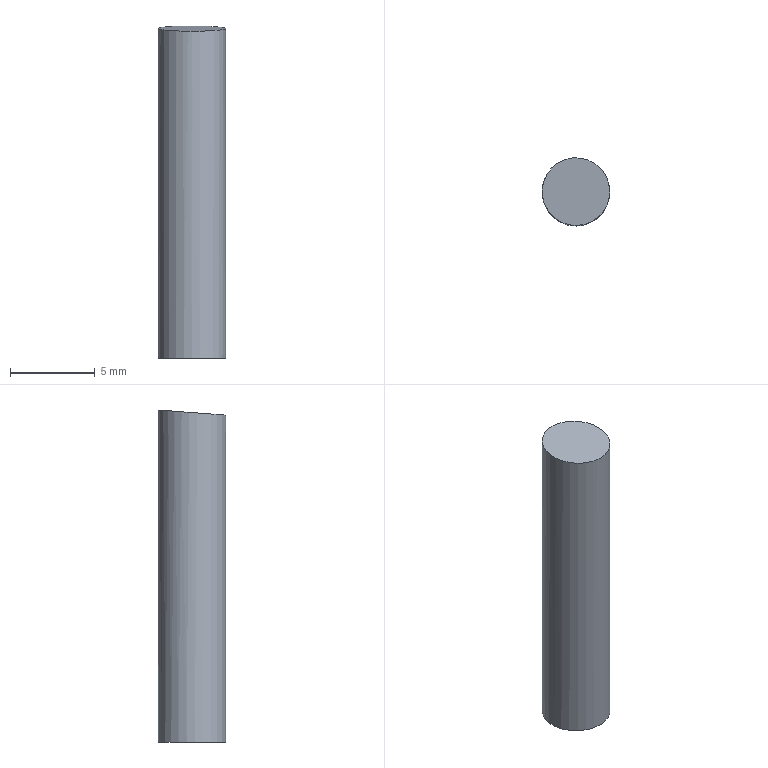Part | NX | features solid 2 | 1 solid | 3 faces | box 4 x 4 x 19.611 mm | volume 244.499 mm3 | plane 2 | cylinder 1 | commonest cylinder face diameters 4 x1
STEP:
#1=CARTESIAN_POINT('',(327.26,-25.675,-35.5));
#2=VERTEX_POINT('',#1);
#3=CARTESIAN_POINT('',(325.26,-25.675,-35.5));
#4=DIRECTION('',(0.,0.,1.));
#5=DIRECTION('',(1.,0.,0.));
#6=AXIS2_PLACEMENT_3D('',#3,#4,#5);
#7=CIRCLE('',#6,2.);
#8=EDGE_CURVE('',#2,#2,#7,.T.);
#9=ORIENTED_EDGE('',*,*,#8,.F.);
#10=EDGE_LOOP('',(#9));
#11=FACE_BOUND('',#10,.T.);
#12=CARTESIAN_POINT('',(325.26,-25.675,-35.5));
#13=DIRECTION('',(0.,0.,-1.));
#14=DIRECTION('',(-1.,0.,0.));
#15=AXIS2_PLACEMENT_3D('',#12,#13,#14);
#16=PLANE('',#15);
#17=ADVANCED_FACE('',(#11),#16,.T.);
#18=CARTESIAN_POINT('',(325.279,-27.675,-16.197));
#19=VERTEX_POINT('',#18);
#20=CARTESIAN_POINT('',(325.26,-25.675,-16.043));
#21=DIRECTION('',(0.0007587,-0.07675,0.9971));
#22=DIRECTION('',(0.009856,-0.997,-0.07675));
#23=AXIS2_PLACEMENT_3D('',#20,#21,#22);
#24=ELLIPSE('',#23,2.006,2.);
#25=EDGE_CURVE('',#19,#19,#24,.F.);
#26=ORIENTED_EDGE('',*,*,#25,.F.);
#27=EDGE_LOOP('',(#26));
#28=FACE_BOUND('',#27,.T.);
#29=CARTESIAN_POINT('',(464.929,116.723,-5.189));
#30=DIRECTION('',(0.0007587,-0.07675,0.9971));
#31=DIRECTION('',(-1.,0.004401,0.0011));
#32=AXIS2_PLACEMENT_3D('',#29,#30,#31);
#33=PLANE('',#32);
#34=ADVANCED_FACE('',(#28),#33,.T.);
#35=ORIENTED_EDGE('',*,*,#8,.T.);
#36=EDGE_LOOP('',(#35));
#37=FACE_BOUND('',#36,.T.);
#38=ORIENTED_EDGE('',*,*,#25,.T.);
#39=EDGE_LOOP('',(#38));
#40=FACE_BOUND('',#39,.T.);
#41=CARTESIAN_POINT('',(325.26,-25.675,-15.5));
#42=DIRECTION('',(0.,0.,-1.));
#43=DIRECTION('',(-1.,0.,0.));
#44=AXIS2_PLACEMENT_3D('',#41,#42,#43);
#45=CYLINDRICAL_SURFACE('',#44,2.);
#46=ADVANCED_FACE('',(#37,#40),#45,.T.);
#47=CLOSED_SHELL('',(#17,#34,#46));
#48=MANIFOLD_SOLID_BREP('',#47);
#49=(LENGTH_UNIT()NAMED_UNIT(*)SI_UNIT(.MILLI.,.METRE.));
#50=UNCERTAINTY_MEASURE_WITH_UNIT(LENGTH_MEASURE(0.00001),#49,'','');
#51=(NAMED_UNIT(*)PLANE_ANGLE_UNIT()SI_UNIT($,.RADIAN.));
#52=(NAMED_UNIT(*)SI_UNIT($,.STERADIAN.)SOLID_ANGLE_UNIT());
#53=(GEOMETRIC_REPRESENTATION_CONTEXT(3)GLOBAL_UNCERTAINTY_ASSIGNED_CONTEXT((#50))GLOBAL_UNIT_ASSIGNED_CONTEXT((#49,#51,#52))REPRESENTATION_CONTEXT('',''));
#54=ADVANCED_BREP_SHAPE_REPRESENTATION('',(#48),#53);